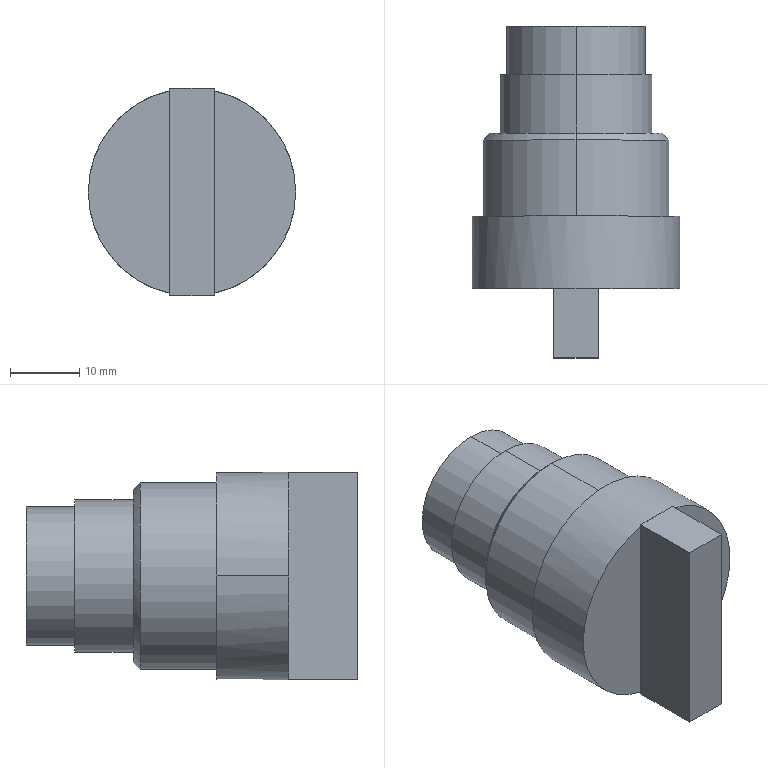Part | SolidWorks | features ICE 2, BaseBody 1 | 1 solid | 28 faces | box 30 x 48 x 30 mm | volume 20868 mm3 | plane 16 | cylinder 10 | cone 2 | commonest cylinder face diameters 18 x2 20 x2 22 x2 27 x2 30 x2
STEP:
#1=CARTESIAN_POINT('',(3.25,8.5,-14.644));
#2=VERTEX_POINT('',#1);
#3=CARTESIAN_POINT('',(3.25,8.5,14.644));
#4=VERTEX_POINT('',#3);
#5=CARTESIAN_POINT('',(3.25,8.5,-15.));
#6=DIRECTION('',(0.,0.,1.));
#7=VECTOR('',#6,1000.);
#8=LINE('',#5,#7);
#9=EDGE_CURVE('',#2,#4,#8,.T.);
#10=ORIENTED_EDGE('',*,*,#9,.F.);
#11=CARTESIAN_POINT('',(15.,8.5,0.));
#12=VERTEX_POINT('',#11);
#13=CARTESIAN_POINT('',(0.,8.5,0.));
#14=DIRECTION('',(0.,1.,0.));
#15=DIRECTION('',(1.,0.,0.));
#16=AXIS2_PLACEMENT_3D('',#13,#14,#15);
#17=CIRCLE('',#16,15.);
#18=EDGE_CURVE('',#12,#2,#17,.T.);
#19=ORIENTED_EDGE('',*,*,#18,.F.);
#20=CARTESIAN_POINT('',(0.,8.5,0.));
#21=DIRECTION('',(0.,1.,0.));
#22=DIRECTION('',(-1.,0.,0.));
#23=AXIS2_PLACEMENT_3D('',#20,#21,#22);
#24=CIRCLE('',#23,15.);
#25=EDGE_CURVE('',#4,#12,#24,.T.);
#26=ORIENTED_EDGE('',*,*,#25,.F.);
#27=EDGE_LOOP('',(#10,#19,#26));
#28=FACE_OUTER_BOUND('',#27,.T.);
#29=CARTESIAN_POINT('',(-24.123,8.5,-20.));
#30=DIRECTION('',(0.,1.,0.));
#31=DIRECTION('',(0.,0.,1.));
#32=AXIS2_PLACEMENT_3D('',#29,#30,#31);
#33=PLANE('',#32);
#34=ADVANCED_FACE('',(#28),#33,.F.);
#35=CARTESIAN_POINT('',(-3.25,8.5,14.644));
#36=VERTEX_POINT('',#35);
#37=CARTESIAN_POINT('',(-3.25,8.5,-14.644));
#38=VERTEX_POINT('',#37);
#39=CARTESIAN_POINT('',(-3.25,8.5,-15.));
#40=DIRECTION('',(0.,0.,-1.));
#41=VECTOR('',#40,1000.);
#42=LINE('',#39,#41);
#43=EDGE_CURVE('',#36,#38,#42,.T.);
#44=ORIENTED_EDGE('',*,*,#43,.F.);
#45=CARTESIAN_POINT('',(-15.,8.5,0.));
#46=VERTEX_POINT('',#45);
#47=CARTESIAN_POINT('',(0.,8.5,0.));
#48=DIRECTION('',(0.,1.,0.));
#49=DIRECTION('',(-1.,0.,0.));
#50=AXIS2_PLACEMENT_3D('',#47,#48,#49);
#51=CIRCLE('',#50,15.);
#52=EDGE_CURVE('',#46,#36,#51,.T.);
#53=ORIENTED_EDGE('',*,*,#52,.F.);
#54=CARTESIAN_POINT('',(0.,8.5,0.));
#55=DIRECTION('',(0.,1.,0.));
#56=DIRECTION('',(1.,0.,0.));
#57=AXIS2_PLACEMENT_3D('',#54,#55,#56);
#58=CIRCLE('',#57,15.);
#59=EDGE_CURVE('',#38,#46,#58,.T.);
#60=ORIENTED_EDGE('',*,*,#59,.F.);
#61=EDGE_LOOP('',(#44,#53,#60));
#62=FACE_OUTER_BOUND('',#61,.T.);
#63=CARTESIAN_POINT('',(-24.123,8.5,-20.));
#64=DIRECTION('',(0.,1.,0.));
#65=DIRECTION('',(0.,0.,1.));
#66=AXIS2_PLACEMENT_3D('',#63,#64,#65);
#67=PLANE('',#66);
#68=ADVANCED_FACE('',(#62),#67,.F.);
#69=CARTESIAN_POINT('',(9.,43.5,0.));
#70=VERTEX_POINT('',#69);
#71=CARTESIAN_POINT('',(-9.,43.5,0.));
#72=VERTEX_POINT('',#71);
#73=CARTESIAN_POINT('',(0.,43.5,0.));
#74=DIRECTION('',(0.,1.,0.));
#75=DIRECTION('',(1.,0.,0.));
#76=AXIS2_PLACEMENT_3D('',#73,#74,#75);
#77=CIRCLE('',#76,9.);
#78=EDGE_CURVE('',#70,#72,#77,.T.);
#79=ORIENTED_EDGE('',*,*,#78,.T.);
#80=CARTESIAN_POINT('',(0.,43.5,0.));
#81=DIRECTION('',(0.,1.,0.));
#82=DIRECTION('',(-1.,0.,0.));
#83=AXIS2_PLACEMENT_3D('',#80,#81,#82);
#84=CIRCLE('',#83,9.);
#85=EDGE_CURVE('',#72,#70,#84,.T.);
#86=ORIENTED_EDGE('',*,*,#85,.T.);
#87=EDGE_LOOP('',(#79,#86));
#88=FACE_OUTER_BOUND('',#87,.T.);
#89=CARTESIAN_POINT('',(0.,43.5,0.));
#90=DIRECTION('',(0.,1.,0.));
#91=DIRECTION('',(-1.,0.,0.));
#92=AXIS2_PLACEMENT_3D('',#89,#90,#91);
#93=PLANE('',#92);
#94=ADVANCED_FACE('',(#88),#93,.T.);
#95=CARTESIAN_POINT('',(-9.,46.5,0.));
#96=VERTEX_POINT('',#95);
#97=CARTESIAN_POINT('',(-9.,46.5,0.));
#98=DIRECTION('',(0.,-1.,0.));
#99=VECTOR('',#98,1000.);
#100=LINE('',#97,#99);
#101=EDGE_CURVE('',#96,#72,#100,.T.);
#102=ORIENTED_EDGE('',*,*,#101,.T.);
#103=ORIENTED_EDGE('',*,*,#78,.F.);
#104=CARTESIAN_POINT('',(9.,46.5,0.));
#105=VERTEX_POINT('',#104);
#106=CARTESIAN_POINT('',(9.,46.5,0.));
#107=DIRECTION('',(0.,-1.,0.));
#108=VECTOR('',#107,1000.);
#109=LINE('',#106,#108);
#110=EDGE_CURVE('',#105,#70,#109,.T.);
#111=ORIENTED_EDGE('',*,*,#110,.F.);
#112=CARTESIAN_POINT('',(0.,46.5,0.));
#113=DIRECTION('',(0.,1.,0.));
#114=DIRECTION('',(1.,0.,0.));
#115=AXIS2_PLACEMENT_3D('',#112,#113,#114);
#116=CIRCLE('',#115,9.);
#117=EDGE_CURVE('',#105,#96,#116,.T.);
#118=ORIENTED_EDGE('',*,*,#117,.T.);
#119=EDGE_LOOP('',(#102,#103,#111,#118));
#120=FACE_OUTER_BOUND('',#119,.T.);
#121=CARTESIAN_POINT('',(0.,46.5,0.));
#122=DIRECTION('',(0.,1.,0.));
#123=DIRECTION('',(-1.,0.,0.));
#124=AXIS2_PLACEMENT_3D('',#121,#122,#123);
#125=CYLINDRICAL_SURFACE('',#124,9.);
#126=ADVANCED_FACE('',(#120),#125,.F.);
#127=ORIENTED_EDGE('',*,*,#110,.T.);
#128=ORIENTED_EDGE('',*,*,#85,.F.);
#129=ORIENTED_EDGE('',*,*,#101,.F.);
#130=CARTESIAN_POINT('',(0.,46.5,0.));
#131=DIRECTION('',(0.,1.,0.));
#132=DIRECTION('',(-1.,0.,0.));
#133=AXIS2_PLACEMENT_3D('',#130,#131,#132);
#134=CIRCLE('',#133,9.);
#135=EDGE_CURVE('',#96,#105,#134,.T.);
#136=ORIENTED_EDGE('',*,*,#135,.T.);
#137=EDGE_LOOP('',(#127,#128,#129,#136));
#138=FACE_OUTER_BOUND('',#137,.T.);
#139=CARTESIAN_POINT('',(0.,46.5,0.));
#140=DIRECTION('',(0.,1.,0.));
#141=DIRECTION('',(-1.,0.,0.));
#142=AXIS2_PLACEMENT_3D('',#139,#140,#141);
#143=CYLINDRICAL_SURFACE('',#142,9.);
#144=ADVANCED_FACE('',(#138),#143,.F.);
#145=ORIENTED_EDGE('',*,*,#117,.F.);
#146=ORIENTED_EDGE('',*,*,#135,.F.);
#147=EDGE_LOOP('',(#145,#146));
#148=FACE_BOUND('',#147,.T.);
#149=CARTESIAN_POINT('',(0.,46.5,10.));
#150=VERTEX_POINT('',#149);
#151=CARTESIAN_POINT('',(0.,46.5,-10.));
#152=VERTEX_POINT('',#151);
#153=CARTESIAN_POINT('',(0.,46.5,0.));
#154=DIRECTION('',(0.,1.,0.));
#155=DIRECTION('',(0.,0.,1.));
#156=AXIS2_PLACEMENT_3D('',#153,#154,#155);
#157=CIRCLE('',#156,10.);
#158=EDGE_CURVE('',#150,#152,#157,.T.);
#159=ORIENTED_EDGE('',*,*,#158,.T.);
#160=CARTESIAN_POINT('',(0.,46.5,0.));
#161=DIRECTION('',(0.,1.,0.));
#162=DIRECTION('',(0.,0.,-1.));
#163=AXIS2_PLACEMENT_3D('',#160,#161,#162);
#164=CIRCLE('',#163,10.);
#165=EDGE_CURVE('',#152,#150,#164,.T.);
#166=ORIENTED_EDGE('',*,*,#165,.T.);
#167=EDGE_LOOP('',(#159,#166));
#168=FACE_OUTER_BOUND('',#167,.T.);
#169=CARTESIAN_POINT('',(0.,46.5,0.));
#170=DIRECTION('',(0.,1.,0.));
#171=DIRECTION('',(0.,0.,-1.));
#172=AXIS2_PLACEMENT_3D('',#169,#170,#171);
#173=PLANE('',#172);
#174=ADVANCED_FACE('',(#148,#168),#173,.T.);
#175=CARTESIAN_POINT('',(0.,39.5,-10.));
#176=VERTEX_POINT('',#175);
#177=CARTESIAN_POINT('',(0.,39.5,-10.));
#178=DIRECTION('',(0.,1.,0.));
#179=VECTOR('',#178,1000.);
#180=LINE('',#177,#179);
#181=EDGE_CURVE('',#176,#152,#180,.T.);
#182=ORIENTED_EDGE('',*,*,#181,.T.);
#183=ORIENTED_EDGE('',*,*,#158,.F.);
#184=CARTESIAN_POINT('',(0.,39.5,10.));
#185=VERTEX_POINT('',#184);
#186=CARTESIAN_POINT('',(0.,39.5,10.));
#187=DIRECTION('',(0.,1.,0.));
#188=VECTOR('',#187,1000.);
#189=LINE('',#186,#188);
#190=EDGE_CURVE('',#185,#150,#189,.T.);
#191=ORIENTED_EDGE('',*,*,#190,.F.);
#192=CARTESIAN_POINT('',(0.,39.5,0.));
#193=DIRECTION('',(0.,1.,0.));
#194=DIRECTION('',(0.,0.,1.));
#195=AXIS2_PLACEMENT_3D('',#192,#193,#194);
#196=CIRCLE('',#195,10.);
#197=EDGE_CURVE('',#185,#176,#196,.T.);
#198=ORIENTED_EDGE('',*,*,#197,.T.);
#199=EDGE_LOOP('',(#182,#183,#191,#198));
#200=FACE_OUTER_BOUND('',#199,.T.);
#201=CARTESIAN_POINT('',(0.,39.5,0.));
#202=DIRECTION('',(0.,1.,0.));
#203=DIRECTION('',(0.,0.,-1.));
#204=AXIS2_PLACEMENT_3D('',#201,#202,#203);
#205=CYLINDRICAL_SURFACE('',#204,10.);
#206=ADVANCED_FACE('',(#200),#205,.T.);
#207=ORIENTED_EDGE('',*,*,#190,.T.);
#208=ORIENTED_EDGE('',*,*,#165,.F.);
#209=ORIENTED_EDGE('',*,*,#181,.F.);
#210=CARTESIAN_POINT('',(0.,39.5,0.));
#211=DIRECTION('',(0.,1.,0.));
#212=DIRECTION('',(0.,0.,-1.));
#213=AXIS2_PLACEMENT_3D('',#210,#211,#212);
#214=CIRCLE('',#213,10.);
#215=EDGE_CURVE('',#176,#185,#214,.T.);
#216=ORIENTED_EDGE('',*,*,#215,.T.);
#217=EDGE_LOOP('',(#207,#208,#209,#216));
#218=FACE_OUTER_BOUND('',#217,.T.);
#219=CARTESIAN_POINT('',(0.,39.5,0.));
#220=DIRECTION('',(0.,1.,0.));
#221=DIRECTION('',(0.,0.,-1.));
#222=AXIS2_PLACEMENT_3D('',#219,#220,#221);
#223=CYLINDRICAL_SURFACE('',#222,10.);
#224=ADVANCED_FACE('',(#218),#223,.T.);
#225=ORIENTED_EDGE('',*,*,#197,.F.);
#226=ORIENTED_EDGE('',*,*,#215,.F.);
#227=EDGE_LOOP('',(#225,#226));
#228=FACE_BOUND('',#227,.T.);
#229=CARTESIAN_POINT('',(0.,39.5,11.));
#230=VERTEX_POINT('',#229);
#231=CARTESIAN_POINT('',(0.,39.5,-11.));
#232=VERTEX_POINT('',#231);
#233=CARTESIAN_POINT('',(0.,39.5,0.));
#234=DIRECTION('',(0.,1.,0.));
#235=DIRECTION('',(0.,0.,1.));
#236=AXIS2_PLACEMENT_3D('',#233,#234,#235);
#237=CIRCLE('',#236,11.);
#238=EDGE_CURVE('',#230,#232,#237,.T.);
#239=ORIENTED_EDGE('',*,*,#238,.T.);
#240=CARTESIAN_POINT('',(0.,39.5,0.));
#241=DIRECTION('',(0.,1.,0.));
#242=DIRECTION('',(0.,0.,-1.));
#243=AXIS2_PLACEMENT_3D('',#240,#241,#242);
#244=CIRCLE('',#243,11.);
#245=EDGE_CURVE('',#232,#230,#244,.T.);
#246=ORIENTED_EDGE('',*,*,#245,.T.);
#247=EDGE_LOOP('',(#239,#246));
#248=FACE_OUTER_BOUND('',#247,.T.);
#249=CARTESIAN_POINT('',(0.,39.5,0.));
#250=DIRECTION('',(0.,1.,0.));
#251=DIRECTION('',(0.,0.,-1.));
#252=AXIS2_PLACEMENT_3D('',#249,#250,#251);
#253=PLANE('',#252);
#254=ADVANCED_FACE('',(#228,#248),#253,.T.);
#255=CARTESIAN_POINT('',(0.,31.,-11.));
#256=VERTEX_POINT('',#255);
#257=CARTESIAN_POINT('',(0.,31.,-11.));
#258=DIRECTION('',(0.,1.,0.));
#259=VECTOR('',#258,1000.);
#260=LINE('',#257,#259);
#261=EDGE_CURVE('',#256,#232,#260,.T.);
#262=ORIENTED_EDGE('',*,*,#261,.T.);
#263=ORIENTED_EDGE('',*,*,#238,.F.);
#264=CARTESIAN_POINT('',(0.,31.,11.));
#265=VERTEX_POINT('',#264);
#266=CARTESIAN_POINT('',(0.,31.,11.));
#267=DIRECTION('',(0.,1.,0.));
#268=VECTOR('',#267,1000.);
#269=LINE('',#266,#268);
#270=EDGE_CURVE('',#265,#230,#269,.T.);
#271=ORIENTED_EDGE('',*,*,#270,.F.);
#272=CARTESIAN_POINT('',(0.,31.,0.));
#273=DIRECTION('',(0.,1.,0.));
#274=DIRECTION('',(0.,0.,1.));
#275=AXIS2_PLACEMENT_3D('',#272,#273,#274);
#276=CIRCLE('',#275,11.);
#277=EDGE_CURVE('',#265,#256,#276,.T.);
#278=ORIENTED_EDGE('',*,*,#277,.T.);
#279=EDGE_LOOP('',(#262,#263,#271,#278));
#280=FACE_OUTER_BOUND('',#279,.T.);
#281=CARTESIAN_POINT('',(0.,31.,0.));
#282=DIRECTION('',(0.,1.,0.));
#283=DIRECTION('',(0.,0.,-1.));
#284=AXIS2_PLACEMENT_3D('',#281,#282,#283);
#285=CYLINDRICAL_SURFACE('',#284,11.);
#286=ADVANCED_FACE('',(#280),#285,.T.);
#287=ORIENTED_EDGE('',*,*,#270,.T.);
#288=ORIENTED_EDGE('',*,*,#245,.F.);
#289=ORIENTED_EDGE('',*,*,#261,.F.);
#290=CARTESIAN_POINT('',(0.,31.,0.));
#291=DIRECTION('',(0.,1.,0.));
#292=DIRECTION('',(0.,0.,-1.));
#293=AXIS2_PLACEMENT_3D('',#290,#291,#292);
#294=CIRCLE('',#293,11.);
#295=EDGE_CURVE('',#256,#265,#294,.T.);
#296=ORIENTED_EDGE('',*,*,#295,.T.);
#297=EDGE_LOOP('',(#287,#288,#289,#296));
#298=FACE_OUTER_BOUND('',#297,.T.);
#299=CARTESIAN_POINT('',(0.,31.,0.));
#300=DIRECTION('',(0.,1.,0.));
#301=DIRECTION('',(0.,0.,-1.));
#302=AXIS2_PLACEMENT_3D('',#299,#300,#301);
#303=CYLINDRICAL_SURFACE('',#302,11.);
#304=ADVANCED_FACE('',(#298),#303,.T.);
#305=CARTESIAN_POINT('',(0.,19.,13.5));
#306=VERTEX_POINT('',#305);
#307=CARTESIAN_POINT('',(0.000000003,30.,13.5));
#308=VERTEX_POINT('',#307);
#309=CARTESIAN_POINT('',(0.,19.,13.5));
#310=DIRECTION('',(0.,1.,0.));
#311=VECTOR('',#310,1000.);
#312=LINE('',#309,#311);
#313=EDGE_CURVE('',#306,#308,#312,.T.);
#314=ORIENTED_EDGE('',*,*,#313,.F.);
#315=CARTESIAN_POINT('',(0.,19.,-13.5));
#316=VERTEX_POINT('',#315);
#317=CARTESIAN_POINT('',(0.,19.,0.));
#318=DIRECTION('',(0.,1.,0.));
#319=DIRECTION('',(0.,0.,1.));
#320=AXIS2_PLACEMENT_3D('',#317,#318,#319);
#321=CIRCLE('',#320,13.5);
#322=EDGE_CURVE('',#306,#316,#321,.T.);
#323=ORIENTED_EDGE('',*,*,#322,.T.);
#324=CARTESIAN_POINT('',(-0.000000003,30.,-13.5));
#325=VERTEX_POINT('',#324);
#326=CARTESIAN_POINT('',(0.,19.,-13.5));
#327=DIRECTION('',(0.,1.,0.));
#328=VECTOR('',#327,1000.);
#329=LINE('',#326,#328);
#330=EDGE_CURVE('',#316,#325,#329,.T.);
#331=ORIENTED_EDGE('',*,*,#330,.T.);
#332=CARTESIAN_POINT('',(0.,30.,0.));
#333=DIRECTION('',(0.,1.,0.));
#334=DIRECTION('',(0.,0.,1.));
#335=AXIS2_PLACEMENT_3D('',#332,#333,#334);
#336=CIRCLE('',#335,13.5);
#337=EDGE_CURVE('',#308,#325,#336,.T.);
#338=ORIENTED_EDGE('',*,*,#337,.F.);
#339=EDGE_LOOP('',(#314,#323,#331,#338));
#340=FACE_OUTER_BOUND('',#339,.T.);
#341=CARTESIAN_POINT('',(0.,19.,0.));
#342=DIRECTION('',(0.,1.,0.));
#343=DIRECTION('',(0.,0.,-1.));
#344=AXIS2_PLACEMENT_3D('',#341,#342,#343);
#345=CYLINDRICAL_SURFACE('',#344,13.5);
#346=ADVANCED_FACE('',(#340),#345,.T.);
#347=CARTESIAN_POINT('',(0.000000004,31.,12.5));
#348=VERTEX_POINT('',#347);
#349=CARTESIAN_POINT('',(-0.00000005,31.,12.5));
#350=DIRECTION('',(-0.000000003,-0.7071,0.7071));
#351=VECTOR('',#350,1000.);
#352=LINE('',#349,#351);
#353=EDGE_CURVE('',#348,#308,#352,.T.);
#354=ORIENTED_EDGE('',*,*,#353,.T.);
#355=ORIENTED_EDGE('',*,*,#337,.T.);
#356=CARTESIAN_POINT('',(-0.000000004,31.,-12.5));
#357=VERTEX_POINT('',#356);
#358=CARTESIAN_POINT('',(0.00000005,31.,-12.5));
#359=DIRECTION('',(0.000000003,-0.7071,-0.7071));
#360=VECTOR('',#359,1000.);
#361=LINE('',#358,#360);
#362=EDGE_CURVE('',#357,#325,#361,.T.);
#363=ORIENTED_EDGE('',*,*,#362,.F.);
#364=CARTESIAN_POINT('',(0.,31.,0.));
#365=DIRECTION('',(0.,1.,0.));
#366=DIRECTION('',(0.,0.,1.));
#367=AXIS2_PLACEMENT_3D('',#364,#365,#366);
#368=CIRCLE('',#367,12.5);
#369=EDGE_CURVE('',#348,#357,#368,.T.);
#370=ORIENTED_EDGE('',*,*,#369,.F.);
#371=EDGE_LOOP('',(#354,#355,#363,#370));
#372=FACE_OUTER_BOUND('',#371,.T.);
#373=CARTESIAN_POINT('',(0.,31.062,0.));
#374=DIRECTION('',(0.,-1.,0.));
#375=DIRECTION('',(0.,0.,-1.));
#376=AXIS2_PLACEMENT_3D('',#373,#374,#375);
#377=CONICAL_SURFACE('',#376,12.438,0.7854);
#378=ADVANCED_FACE('',(#372),#377,.T.);
#379=ORIENTED_EDGE('',*,*,#277,.F.);
#380=ORIENTED_EDGE('',*,*,#295,.F.);
#381=EDGE_LOOP('',(#379,#380));
#382=FACE_BOUND('',#381,.T.);
#383=CARTESIAN_POINT('',(0.,31.,0.));
#384=DIRECTION('',(0.,1.,0.));
#385=DIRECTION('',(0.,0.,-1.));
#386=AXIS2_PLACEMENT_3D('',#383,#384,#385);
#387=CIRCLE('',#386,12.5);
#388=EDGE_CURVE('',#357,#348,#387,.T.);
#389=ORIENTED_EDGE('',*,*,#388,.T.);
#390=ORIENTED_EDGE('',*,*,#369,.T.);
#391=EDGE_LOOP('',(#389,#390));
#392=FACE_OUTER_BOUND('',#391,.T.);
#393=CARTESIAN_POINT('',(0.,31.,0.));
#394=DIRECTION('',(0.,1.,0.));
#395=DIRECTION('',(0.,0.,-1.));
#396=AXIS2_PLACEMENT_3D('',#393,#394,#395);
#397=PLANE('',#396);
#398=ADVANCED_FACE('',(#382,#392),#397,.T.);
#399=ORIENTED_EDGE('',*,*,#362,.T.);
#400=CARTESIAN_POINT('',(0.,30.,0.));
#401=DIRECTION('',(0.,1.,0.));
#402=DIRECTION('',(0.,0.,-1.));
#403=AXIS2_PLACEMENT_3D('',#400,#401,#402);
#404=CIRCLE('',#403,13.5);
#405=EDGE_CURVE('',#325,#308,#404,.T.);
#406=ORIENTED_EDGE('',*,*,#405,.T.);
#407=ORIENTED_EDGE('',*,*,#353,.F.);
#408=ORIENTED_EDGE('',*,*,#388,.F.);
#409=EDGE_LOOP('',(#399,#406,#407,#408));
#410=FACE_OUTER_BOUND('',#409,.T.);
#411=CARTESIAN_POINT('',(0.,31.062,0.));
#412=DIRECTION('',(0.,-1.,0.));
#413=DIRECTION('',(0.,0.,-1.));
#414=AXIS2_PLACEMENT_3D('',#411,#412,#413);
#415=CONICAL_SURFACE('',#414,12.438,0.7854);
#416=ADVANCED_FACE('',(#410),#415,.T.);
#417=ORIENTED_EDGE('',*,*,#330,.F.);
#418=CARTESIAN_POINT('',(0.,19.,0.));
#419=DIRECTION('',(0.,1.,0.));
#420=DIRECTION('',(0.,0.,-1.));
#421=AXIS2_PLACEMENT_3D('',#418,#419,#420);
#422=CIRCLE('',#421,13.5);
#423=EDGE_CURVE('',#316,#306,#422,.T.);
#424=ORIENTED_EDGE('',*,*,#423,.T.);
#425=ORIENTED_EDGE('',*,*,#313,.T.);
#426=ORIENTED_EDGE('',*,*,#405,.F.);
#427=EDGE_LOOP('',(#417,#424,#425,#426));
#428=FACE_OUTER_BOUND('',#427,.T.);
#429=CARTESIAN_POINT('',(0.,19.,0.));
#430=DIRECTION('',(0.,1.,0.));
#431=DIRECTION('',(0.,0.,-1.));
#432=AXIS2_PLACEMENT_3D('',#429,#430,#431);
#433=CYLINDRICAL_SURFACE('',#432,13.5);
#434=ADVANCED_FACE('',(#428),#433,.T.);
#435=ORIENTED_EDGE('',*,*,#322,.F.);
#436=ORIENTED_EDGE('',*,*,#423,.F.);
#437=EDGE_LOOP('',(#435,#436));
#438=FACE_BOUND('',#437,.T.);
#439=CARTESIAN_POINT('',(-15.,19.,0.));
#440=VERTEX_POINT('',#439);
#441=CARTESIAN_POINT('',(15.,19.,0.));
#442=VERTEX_POINT('',#441);
#443=CARTESIAN_POINT('',(0.,19.,0.));
#444=DIRECTION('',(0.,1.,0.));
#445=DIRECTION('',(-1.,0.,0.));
#446=AXIS2_PLACEMENT_3D('',#443,#444,#445);
#447=CIRCLE('',#446,15.);
#448=EDGE_CURVE('',#440,#442,#447,.T.);
#449=ORIENTED_EDGE('',*,*,#448,.T.);
#450=CARTESIAN_POINT('',(0.,19.,0.));
#451=DIRECTION('',(0.,1.,0.));
#452=DIRECTION('',(1.,0.,0.));
#453=AXIS2_PLACEMENT_3D('',#450,#451,#452);
#454=CIRCLE('',#453,15.);
#455=EDGE_CURVE('',#442,#440,#454,.T.);
#456=ORIENTED_EDGE('',*,*,#455,.T.);
#457=EDGE_LOOP('',(#449,#456));
#458=FACE_OUTER_BOUND('',#457,.T.);
#459=CARTESIAN_POINT('',(0.,19.,0.));
#460=DIRECTION('',(0.,1.,0.));
#461=DIRECTION('',(1.,0.,0.));
#462=AXIS2_PLACEMENT_3D('',#459,#460,#461);
#463=PLANE('',#462);
#464=ADVANCED_FACE('',(#438,#458),#463,.T.);
#465=CARTESIAN_POINT('',(15.,8.5,0.));
#466=DIRECTION('',(0.,1.,0.));
#467=VECTOR('',#466,1000.);
#468=LINE('',#465,#467);
#469=EDGE_CURVE('',#12,#442,#468,.T.);
#470=ORIENTED_EDGE('',*,*,#469,.T.);
#471=ORIENTED_EDGE('',*,*,#448,.F.);
#472=CARTESIAN_POINT('',(-15.,8.5,0.));
#473=DIRECTION('',(0.,1.,0.));
#474=VECTOR('',#473,1000.);
#475=LINE('',#472,#474);
#476=EDGE_CURVE('',#46,#440,#475,.T.);
#477=ORIENTED_EDGE('',*,*,#476,.F.);
#478=ORIENTED_EDGE('',*,*,#52,.T.);
#479=CARTESIAN_POINT('',(0.,8.5,15.));
#480=VERTEX_POINT('',#479);
#481=CARTESIAN_POINT('',(0.,8.5,0.));
#482=DIRECTION('',(0.,1.,0.));
#483=DIRECTION('',(-1.,0.,0.));
#484=AXIS2_PLACEMENT_3D('',#481,#482,#483);
#485=CIRCLE('',#484,15.);
#486=EDGE_CURVE('',#36,#480,#485,.T.);
#487=ORIENTED_EDGE('',*,*,#486,.T.);
#488=CARTESIAN_POINT('',(0.,8.5,0.));
#489=DIRECTION('',(0.,1.,0.));
#490=DIRECTION('',(-1.,0.,0.));
#491=AXIS2_PLACEMENT_3D('',#488,#489,#490);
#492=CIRCLE('',#491,15.);
#493=EDGE_CURVE('',#480,#4,#492,.T.);
#494=ORIENTED_EDGE('',*,*,#493,.T.);
#495=ORIENTED_EDGE('',*,*,#25,.T.);
#496=EDGE_LOOP('',(#470,#471,#477,#478,#487,#494,#495));
#497=FACE_OUTER_BOUND('',#496,.T.);
#498=CARTESIAN_POINT('',(0.,6.,0.));
#499=DIRECTION('',(0.,1.,0.));
#500=DIRECTION('',(1.,0.,0.));
#501=AXIS2_PLACEMENT_3D('',#498,#499,#500);
#502=CYLINDRICAL_SURFACE('',#501,15.);
#503=ADVANCED_FACE('',(#497),#502,.T.);
#504=ORIENTED_EDGE('',*,*,#476,.T.);
#505=ORIENTED_EDGE('',*,*,#455,.F.);
#506=ORIENTED_EDGE('',*,*,#469,.F.);
#507=ORIENTED_EDGE('',*,*,#18,.T.);
#508=CARTESIAN_POINT('',(0.,8.5,-15.));
#509=VERTEX_POINT('',#508);
#510=CARTESIAN_POINT('',(0.,8.5,0.));
#511=DIRECTION('',(0.,1.,0.));
#512=DIRECTION('',(1.,0.,0.));
#513=AXIS2_PLACEMENT_3D('',#510,#511,#512);
#514=CIRCLE('',#513,15.);
#515=EDGE_CURVE('',#2,#509,#514,.T.);
#516=ORIENTED_EDGE('',*,*,#515,.T.);
#517=CARTESIAN_POINT('',(0.,8.5,0.));
#518=DIRECTION('',(0.,1.,0.));
#519=DIRECTION('',(1.,0.,0.));
#520=AXIS2_PLACEMENT_3D('',#517,#518,#519);
#521=CIRCLE('',#520,15.);
#522=EDGE_CURVE('',#509,#38,#521,.T.);
#523=ORIENTED_EDGE('',*,*,#522,.T.);
#524=ORIENTED_EDGE('',*,*,#59,.T.);
#525=EDGE_LOOP('',(#504,#505,#506,#507,#516,#523,#524));
#526=FACE_OUTER_BOUND('',#525,.T.);
#527=CARTESIAN_POINT('',(0.,6.,0.));
#528=DIRECTION('',(0.,1.,0.));
#529=DIRECTION('',(1.,0.,0.));
#530=AXIS2_PLACEMENT_3D('',#527,#528,#529);
#531=CYLINDRICAL_SURFACE('',#530,15.);
#532=ADVANCED_FACE('',(#526),#531,.T.);
#533=ORIENTED_EDGE('',*,*,#486,.F.);
#534=CARTESIAN_POINT('',(-3.25,8.5,15.));
#535=VERTEX_POINT('',#534);
#536=CARTESIAN_POINT('',(-3.25,8.5,-15.));
#537=DIRECTION('',(0.,0.,-1.));
#538=VECTOR('',#537,1000.);
#539=LINE('',#536,#538);
#540=EDGE_CURVE('',#535,#36,#539,.T.);
#541=ORIENTED_EDGE('',*,*,#540,.F.);
#542=CARTESIAN_POINT('',(-3.25,8.5,15.));
#543=DIRECTION('',(-1.,0.,0.));
#544=VECTOR('',#543,1000.);
#545=LINE('',#542,#544);
#546=EDGE_CURVE('',#480,#535,#545,.T.);
#547=ORIENTED_EDGE('',*,*,#546,.F.);
#548=EDGE_LOOP('',(#533,#541,#547));
#549=FACE_OUTER_BOUND('',#548,.T.);
#550=CARTESIAN_POINT('',(0.,8.5,0.));
#551=DIRECTION('',(0.,1.,0.));
#552=DIRECTION('',(0.,0.,1.));
#553=AXIS2_PLACEMENT_3D('',#550,#551,#552);
#554=PLANE('',#553);
#555=ADVANCED_FACE('',(#549),#554,.T.);
#556=ORIENTED_EDGE('',*,*,#493,.F.);
#557=CARTESIAN_POINT('',(3.25,8.5,15.));
#558=VERTEX_POINT('',#557);
#559=CARTESIAN_POINT('',(-3.25,8.5,15.));
#560=DIRECTION('',(-1.,0.,0.));
#561=VECTOR('',#560,1000.);
#562=LINE('',#559,#561);
#563=EDGE_CURVE('',#558,#480,#562,.T.);
#564=ORIENTED_EDGE('',*,*,#563,.F.);
#565=CARTESIAN_POINT('',(3.25,8.5,-15.));
#566=DIRECTION('',(0.,0.,1.));
#567=VECTOR('',#566,1000.);
#568=LINE('',#565,#567);
#569=EDGE_CURVE('',#4,#558,#568,.T.);
#570=ORIENTED_EDGE('',*,*,#569,.F.);
#571=EDGE_LOOP('',(#556,#564,#570));
#572=FACE_OUTER_BOUND('',#571,.T.);
#573=CARTESIAN_POINT('',(0.,8.5,0.));
#574=DIRECTION('',(0.,1.,0.));
#575=DIRECTION('',(0.,0.,1.));
#576=AXIS2_PLACEMENT_3D('',#573,#574,#575);
#577=PLANE('',#576);
#578=ADVANCED_FACE('',(#572),#577,.T.);
#579=ORIENTED_EDGE('',*,*,#515,.F.);
#580=CARTESIAN_POINT('',(3.25,8.5,-15.));
#581=VERTEX_POINT('',#580);
#582=CARTESIAN_POINT('',(3.25,8.5,-15.));
#583=DIRECTION('',(0.,0.,1.));
#584=VECTOR('',#583,1000.);
#585=LINE('',#582,#584);
#586=EDGE_CURVE('',#581,#2,#585,.T.);
#587=ORIENTED_EDGE('',*,*,#586,.F.);
#588=CARTESIAN_POINT('',(-3.25,8.5,-15.));
#589=DIRECTION('',(1.,0.,0.));
#590=VECTOR('',#589,1000.);
#591=LINE('',#588,#590);
#592=EDGE_CURVE('',#509,#581,#591,.T.);
#593=ORIENTED_EDGE('',*,*,#592,.F.);
#594=EDGE_LOOP('',(#579,#587,#593));
#595=FACE_OUTER_BOUND('',#594,.T.);
#596=CARTESIAN_POINT('',(0.,8.5,0.));
#597=DIRECTION('',(0.,1.,0.));
#598=DIRECTION('',(0.,0.,1.));
#599=AXIS2_PLACEMENT_3D('',#596,#597,#598);
#600=PLANE('',#599);
#601=ADVANCED_FACE('',(#595),#600,.T.);
#602=ORIENTED_EDGE('',*,*,#522,.F.);
#603=CARTESIAN_POINT('',(-3.25,8.5,-15.));
#604=VERTEX_POINT('',#603);
#605=CARTESIAN_POINT('',(-3.25,8.5,-15.));
#606=DIRECTION('',(1.,0.,0.));
#607=VECTOR('',#606,1000.);
#608=LINE('',#605,#607);
#609=EDGE_CURVE('',#604,#509,#608,.T.);
#610=ORIENTED_EDGE('',*,*,#609,.F.);
#611=CARTESIAN_POINT('',(-3.25,8.5,-15.));
#612=DIRECTION('',(0.,0.,-1.));
#613=VECTOR('',#612,1000.);
#614=LINE('',#611,#613);
#615=EDGE_CURVE('',#38,#604,#614,.T.);
#616=ORIENTED_EDGE('',*,*,#615,.F.);
#617=EDGE_LOOP('',(#602,#610,#616));
#618=FACE_OUTER_BOUND('',#617,.T.);
#619=CARTESIAN_POINT('',(0.,8.5,0.));
#620=DIRECTION('',(0.,1.,0.));
#621=DIRECTION('',(0.,0.,1.));
#622=AXIS2_PLACEMENT_3D('',#619,#620,#621);
#623=PLANE('',#622);
#624=ADVANCED_FACE('',(#618),#623,.T.);
#625=ORIENTED_EDGE('',*,*,#586,.T.);
#626=ORIENTED_EDGE('',*,*,#9,.T.);
#627=ORIENTED_EDGE('',*,*,#569,.T.);
#628=CARTESIAN_POINT('',(3.25,-1.5,15.));
#629=VERTEX_POINT('',#628);
#630=CARTESIAN_POINT('',(3.25,-1.5,15.));
#631=DIRECTION('',(0.,1.,0.));
#632=VECTOR('',#631,1000.);
#633=LINE('',#630,#632);
#634=EDGE_CURVE('',#629,#558,#633,.T.);
#635=ORIENTED_EDGE('',*,*,#634,.F.);
#636=CARTESIAN_POINT('',(3.25,-1.5,-15.));
#637=VERTEX_POINT('',#636);
#638=CARTESIAN_POINT('',(3.25,-1.5,-15.));
#639=DIRECTION('',(0.,0.,1.));
#640=VECTOR('',#639,1000.);
#641=LINE('',#638,#640);
#642=EDGE_CURVE('',#637,#629,#641,.T.);
#643=ORIENTED_EDGE('',*,*,#642,.F.);
#644=CARTESIAN_POINT('',(3.25,-1.5,-15.));
#645=DIRECTION('',(0.,1.,0.));
#646=VECTOR('',#645,1000.);
#647=LINE('',#644,#646);
#648=EDGE_CURVE('',#637,#581,#647,.T.);
#649=ORIENTED_EDGE('',*,*,#648,.T.);
#650=EDGE_LOOP('',(#625,#626,#627,#635,#643,#649));
#651=FACE_OUTER_BOUND('',#650,.T.);
#652=CARTESIAN_POINT('',(3.25,-1.5,-15.));
#653=DIRECTION('',(-1.,0.,0.));
#654=DIRECTION('',(0.,0.,1.));
#655=AXIS2_PLACEMENT_3D('',#652,#653,#654);
#656=PLANE('',#655);
#657=ADVANCED_FACE('',(#651),#656,.F.);
#658=ORIENTED_EDGE('',*,*,#563,.T.);
#659=ORIENTED_EDGE('',*,*,#546,.T.);
#660=CARTESIAN_POINT('',(-3.25,-1.5,15.));
#661=VERTEX_POINT('',#660);
#662=CARTESIAN_POINT('',(-3.25,-1.5,15.));
#663=DIRECTION('',(0.,1.,0.));
#664=VECTOR('',#663,1000.);
#665=LINE('',#662,#664);
#666=EDGE_CURVE('',#661,#535,#665,.T.);
#667=ORIENTED_EDGE('',*,*,#666,.F.);
#668=CARTESIAN_POINT('',(-3.25,-1.5,15.));
#669=DIRECTION('',(-1.,0.,0.));
#670=VECTOR('',#669,1000.);
#671=LINE('',#668,#670);
#672=EDGE_CURVE('',#629,#661,#671,.T.);
#673=ORIENTED_EDGE('',*,*,#672,.F.);
#674=ORIENTED_EDGE('',*,*,#634,.T.);
#675=EDGE_LOOP('',(#658,#659,#667,#673,#674));
#676=FACE_OUTER_BOUND('',#675,.T.);
#677=CARTESIAN_POINT('',(-3.25,-1.5,15.));
#678=DIRECTION('',(0.,0.,-1.));
#679=DIRECTION('',(-1.,0.,0.));
#680=AXIS2_PLACEMENT_3D('',#677,#678,#679);
#681=PLANE('',#680);
#682=ADVANCED_FACE('',(#676),#681,.F.);
#683=ORIENTED_EDGE('',*,*,#540,.T.);
#684=ORIENTED_EDGE('',*,*,#43,.T.);
#685=ORIENTED_EDGE('',*,*,#615,.T.);
#686=CARTESIAN_POINT('',(-3.25,-1.5,-15.));
#687=VERTEX_POINT('',#686);
#688=CARTESIAN_POINT('',(-3.25,-1.5,-15.));
#689=DIRECTION('',(0.,1.,0.));
#690=VECTOR('',#689,1000.);
#691=LINE('',#688,#690);
#692=EDGE_CURVE('',#687,#604,#691,.T.);
#693=ORIENTED_EDGE('',*,*,#692,.F.);
#694=CARTESIAN_POINT('',(-3.25,-1.5,-15.));
#695=DIRECTION('',(0.,0.,-1.));
#696=VECTOR('',#695,1000.);
#697=LINE('',#694,#696);
#698=EDGE_CURVE('',#661,#687,#697,.T.);
#699=ORIENTED_EDGE('',*,*,#698,.F.);
#700=ORIENTED_EDGE('',*,*,#666,.T.);
#701=EDGE_LOOP('',(#683,#684,#685,#693,#699,#700));
#702=FACE_OUTER_BOUND('',#701,.T.);
#703=CARTESIAN_POINT('',(-3.25,-1.5,-15.));
#704=DIRECTION('',(1.,0.,0.));
#705=DIRECTION('',(0.,0.,-1.));
#706=AXIS2_PLACEMENT_3D('',#703,#704,#705);
#707=PLANE('',#706);
#708=ADVANCED_FACE('',(#702),#707,.F.);
#709=ORIENTED_EDGE('',*,*,#609,.T.);
#710=ORIENTED_EDGE('',*,*,#592,.T.);
#711=ORIENTED_EDGE('',*,*,#648,.F.);
#712=CARTESIAN_POINT('',(-3.25,-1.5,-15.));
#713=DIRECTION('',(1.,0.,0.));
#714=VECTOR('',#713,1000.);
#715=LINE('',#712,#714);
#716=EDGE_CURVE('',#687,#637,#715,.T.);
#717=ORIENTED_EDGE('',*,*,#716,.F.);
#718=ORIENTED_EDGE('',*,*,#692,.T.);
#719=EDGE_LOOP('',(#709,#710,#711,#717,#718));
#720=FACE_OUTER_BOUND('',#719,.T.);
#721=CARTESIAN_POINT('',(-3.25,-1.5,-15.));
#722=DIRECTION('',(0.,0.,1.));
#723=DIRECTION('',(1.,0.,0.));
#724=AXIS2_PLACEMENT_3D('',#721,#722,#723);
#725=PLANE('',#724);
#726=ADVANCED_FACE('',(#720),#725,.F.);
#727=ORIENTED_EDGE('',*,*,#642,.T.);
#728=ORIENTED_EDGE('',*,*,#672,.T.);
#729=ORIENTED_EDGE('',*,*,#698,.T.);
#730=ORIENTED_EDGE('',*,*,#716,.T.);
#731=EDGE_LOOP('',(#727,#728,#729,#730));
#732=FACE_OUTER_BOUND('',#731,.T.);
#733=CARTESIAN_POINT('',(0.,-1.5,0.));
#734=DIRECTION('',(0.,1.,0.));
#735=DIRECTION('',(0.,0.,1.));
#736=AXIS2_PLACEMENT_3D('',#733,#734,#735);
#737=PLANE('',#736);
#738=ADVANCED_FACE('',(#732),#737,.F.);
#739=CLOSED_SHELL('',(#34,#68,#94,#126,#144,#174,#206,#224,#254,#286,#304,#346,#378,#398,#416,#434,#464,#503,#532,#555,#578,#601,#624,#657,#682,#708,#726,#738));
#740=MANIFOLD_SOLID_BREP('',#739);
#741=CARTESIAN_POINT('',(0.,0.,0.));
#742=DIRECTION('',(0.,0.,1.));
#743=DIRECTION('',(1.,0.,0.));
#744=AXIS2_PLACEMENT_3D('',#741,#742,#743);
#745=(LENGTH_UNIT()NAMED_UNIT(*)SI_UNIT(.MILLI.,.METRE.));
#746=UNCERTAINTY_MEASURE_WITH_UNIT(LENGTH_MEASURE(0.00001),#745,'','');
#747=(NAMED_UNIT(*)PLANE_ANGLE_UNIT()SI_UNIT($,.RADIAN.));
#748=(NAMED_UNIT(*)SI_UNIT($,.STERADIAN.)SOLID_ANGLE_UNIT());
#749=(GEOMETRIC_REPRESENTATION_CONTEXT(3)GLOBAL_UNCERTAINTY_ASSIGNED_CONTEXT((#746))GLOBAL_UNIT_ASSIGNED_CONTEXT((#745,#747,#748))REPRESENTATION_CONTEXT('',''));
#750=ADVANCED_BREP_SHAPE_REPRESENTATION('',(#740,#744),#749);